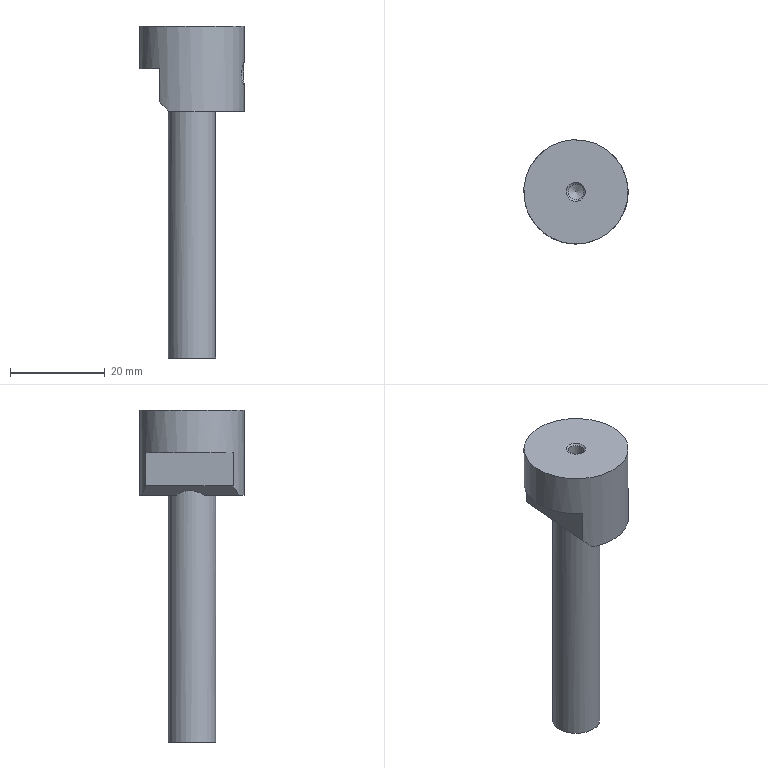Part | STEP file | SL2-MOLD_id358_xmt_txt | 1 solid | 14 faces | box 22 x 22 x 70 mm | volume 6058 mm3 | plane 7 | cylinder 5 | cone 2 | commonest cylinder face diameters 3.3 x1 5 x1 9 x1 10 x1 22 x1
STEP:
#1=CARTESIAN_POINT('',(-61.174,-74.293,77.));
#2=VERTEX_POINT('',#1);
#3=CARTESIAN_POINT('',(-61.174,-74.293,84.));
#4=VERTEX_POINT('',#3);
#5=CARTESIAN_POINT('',(-61.174,-74.293,90.));
#6=DIRECTION('',(0.,0.,1.));
#7=VECTOR('',#6,1.);
#8=LINE('',#5,#7);
#9=EDGE_CURVE('',#2,#4,#8,.T.);
#10=ORIENTED_EDGE('',*,*,#9,.F.);
#11=CARTESIAN_POINT('',(-62.781,-92.662,77.));
#12=VERTEX_POINT('',#11);
#13=CARTESIAN_POINT('',(-62.781,-92.662,77.));
#14=DIRECTION('',(-0.08716,-0.9962,0.));
#15=VECTOR('',#14,1.);
#16=LINE('',#13,#15);
#17=EDGE_CURVE('',#2,#12,#16,.T.);
#18=ORIENTED_EDGE('',*,*,#17,.T.);
#19=CARTESIAN_POINT('',(-62.781,-92.662,84.));
#20=VERTEX_POINT('',#19);
#21=CARTESIAN_POINT('',(-62.781,-92.662,90.));
#22=DIRECTION('',(0.,0.,-1.));
#23=VECTOR('',#22,1.);
#24=LINE('',#21,#23);
#25=EDGE_CURVE('',#20,#12,#24,.T.);
#26=ORIENTED_EDGE('',*,*,#25,.F.);
#27=CARTESIAN_POINT('',(-61.977,-83.477,84.));
#28=DIRECTION('',(-0.08716,-0.9962,0.));
#29=VECTOR('',#28,1.);
#30=LINE('',#27,#29);
#31=EDGE_CURVE('',#4,#20,#30,.T.);
#32=ORIENTED_EDGE('',*,*,#31,.F.);
#33=EDGE_LOOP('',(#10,#18,#26,#32));
#34=FACE_OUTER_BOUND('',#33,.T.);
#35=CARTESIAN_POINT('',(-61.977,-83.477,90.));
#36=DIRECTION('',(-0.9962,0.08716,0.));
#37=DIRECTION('',(0.,0.,-1.));
#38=AXIS2_PLACEMENT_3D('',#35,#36,#37);
#39=PLANE('',#38);
#40=ADVANCED_FACE('',(#34),#39,.T.);
#41=CARTESIAN_POINT('',(-59.092,-73.443,75.));
#42=VERTEX_POINT('',#41);
#43=CARTESIAN_POINT('',(-60.878,-93.859,75.));
#44=VERTEX_POINT('',#43);
#45=CARTESIAN_POINT('',(-56.,-84.,75.));
#46=DIRECTION('',(0.,0.,-1.));
#47=DIRECTION('',(-0.9962,0.08716,0.));
#48=AXIS2_PLACEMENT_3D('',#45,#46,#47);
#49=CIRCLE('',#48,11.);
#50=EDGE_CURVE('',#42,#44,#49,.T.);
#51=ORIENTED_EDGE('',*,*,#50,.T.);
#52=CARTESIAN_POINT('',(-60.246,-86.64,75.));
#53=VERTEX_POINT('',#52);
#54=CARTESIAN_POINT('',(-59.985,-83.651,75.));
#55=DIRECTION('',(0.08716,0.9962,0.));
#56=VECTOR('',#55,1.);
#57=LINE('',#54,#56);
#58=EDGE_CURVE('',#44,#53,#57,.T.);
#59=ORIENTED_EDGE('',*,*,#58,.T.);
#60=CARTESIAN_POINT('',(-59.723,-80.663,75.));
#61=VERTEX_POINT('',#60);
#62=CARTESIAN_POINT('',(-56.,-84.,75.));
#63=DIRECTION('',(0.,0.,1.));
#64=DIRECTION('',(-0.9962,0.08716,0.));
#65=AXIS2_PLACEMENT_3D('',#62,#63,#64);
#66=CIRCLE('',#65,5.);
#67=EDGE_CURVE('',#53,#61,#66,.T.);
#68=ORIENTED_EDGE('',*,*,#67,.T.);
#69=CARTESIAN_POINT('',(-59.985,-83.651,75.));
#70=DIRECTION('',(0.08716,0.9962,0.));
#71=VECTOR('',#70,1.);
#72=LINE('',#69,#71);
#73=EDGE_CURVE('',#61,#42,#72,.T.);
#74=ORIENTED_EDGE('',*,*,#73,.T.);
#75=EDGE_LOOP('',(#51,#59,#68,#74));
#76=FACE_OUTER_BOUND('',#75,.T.);
#77=CARTESIAN_POINT('',(-56.,-84.,75.));
#78=DIRECTION('',(0.,0.,1.));
#79=DIRECTION('',(-0.9962,0.08716,0.));
#80=AXIS2_PLACEMENT_3D('',#77,#78,#79);
#81=PLANE('',#80);
#82=ADVANCED_FACE('',(#76),#81,.F.);
#83=CARTESIAN_POINT('',(-45.115,-85.59,80.582));
#84=VERTEX_POINT('',#83);
#85=CARTESIAN_POINT('',(-45.115,-85.59,80.582));
#86=CARTESIAN_POINT('',(-45.077,-85.328,80.513));
#87=CARTESIAN_POINT('',(-45.047,-85.049,80.487));
#88=CARTESIAN_POINT('',(-45.027,-84.777,80.507));
#89=CARTESIAN_POINT('',(-45.008,-84.505,80.527));
#90=CARTESIAN_POINT('',(-45.,-84.231,80.593));
#91=CARTESIAN_POINT('',(-45.,-83.979,80.7));
#92=CARTESIAN_POINT('',(-45.,-83.726,80.807));
#93=CARTESIAN_POINT('',(-45.01,-83.488,80.958));
#94=CARTESIAN_POINT('',(-45.023,-83.282,81.141));
#95=CARTESIAN_POINT('',(-45.037,-83.073,81.328));
#96=CARTESIAN_POINT('',(-45.055,-82.892,81.553));
#97=CARTESIAN_POINT('',(-45.071,-82.756,81.798));
#98=CARTESIAN_POINT('',(-45.086,-82.618,82.045));
#99=CARTESIAN_POINT('',(-45.1,-82.522,82.32));
#100=CARTESIAN_POINT('',(-45.106,-82.476,82.599));
#101=CARTESIAN_POINT('',(-45.112,-82.431,82.872));
#102=CARTESIAN_POINT('',(-45.112,-82.433,83.157));
#103=CARTESIAN_POINT('',(-45.105,-82.481,83.43));
#104=CARTESIAN_POINT('',(-45.099,-82.529,83.698));
#105=CARTESIAN_POINT('',(-45.086,-82.623,83.962));
#106=CARTESIAN_POINT('',(-45.071,-82.755,84.2));
#107=CARTESIAN_POINT('',(-45.055,-82.889,84.442));
#108=CARTESIAN_POINT('',(-45.038,-83.066,84.664));
#109=CARTESIAN_POINT('',(-45.024,-83.271,84.849));
#110=CARTESIAN_POINT('',(-45.01,-83.481,85.038));
#111=CARTESIAN_POINT('',(-45.,-83.726,85.194));
#112=CARTESIAN_POINT('',(-45.,-83.987,85.303));
#113=CARTESIAN_POINT('',(-45.,-84.246,85.412));
#114=CARTESIAN_POINT('',(-45.009,-84.528,85.478));
#115=CARTESIAN_POINT('',(-45.03,-84.808,85.495));
#116=CARTESIAN_POINT('',(-45.05,-85.082,85.512));
#117=CARTESIAN_POINT('',(-45.081,-85.362,85.482));
#118=CARTESIAN_POINT('',(-45.121,-85.624,85.409));
#119=CARTESIAN_POINT('',(-45.16,-85.885,85.335));
#120=CARTESIAN_POINT('',(-45.207,-86.135,85.217));
#121=CARTESIAN_POINT('',(-45.255,-86.357,85.064));
#122=CARTESIAN_POINT('',(-45.305,-86.582,84.907));
#123=CARTESIAN_POINT('',(-45.357,-86.783,84.71));
#124=CARTESIAN_POINT('',(-45.401,-86.944,84.487));
#125=CARTESIAN_POINT('',(-45.447,-87.109,84.261));
#126=CARTESIAN_POINT('',(-45.487,-87.236,84.002));
#127=CARTESIAN_POINT('',(-45.512,-87.317,83.732));
#128=CARTESIAN_POINT('',(-45.537,-87.397,83.465));
#129=CARTESIAN_POINT('',(-45.549,-87.433,83.179));
#130=CARTESIAN_POINT('',(-45.546,-87.422,82.899));
#131=CARTESIAN_POINT('',(-45.542,-87.411,82.626));
#132=CARTESIAN_POINT('',(-45.524,-87.355,82.351));
#133=CARTESIAN_POINT('',(-45.494,-87.259,82.097));
#134=CARTESIAN_POINT('',(-45.464,-87.163,81.842));
#135=CARTESIAN_POINT('',(-45.422,-87.023,81.601));
#136=CARTESIAN_POINT('',(-45.376,-86.851,81.392));
#137=CARTESIAN_POINT('',(-45.329,-86.675,81.178));
#138=CARTESIAN_POINT('',(-45.276,-86.46,80.993));
#139=CARTESIAN_POINT('',(-45.227,-86.223,80.85));
#140=CARTESIAN_POINT('',(-45.187,-86.027,80.732));
#141=CARTESIAN_POINT('',(-45.148,-85.812,80.641));
#142=CARTESIAN_POINT('',(-45.115,-85.59,80.582));
#143=B_SPLINE_CURVE_WITH_KNOTS('',3,(#85,#86,#87,#88,#89,#90,#91,#92,#93,#94,#95,#96,#97,#98,#99,#100,#101,#102,#103,#104,#105,#106,#107,#108,#109,#110,#111,#112,#113,#114,#115,#116,#117,#118,#119,#120,#121,#122,#123,#124,#125,#126,#127,#128,#129,#130,#131,#132,#133,#134,#135,#136,#137,#138,#139,#140,#141,#142),.UNSPECIFIED.,.T.,.F.,(1,3,3,3,3,3,3,3,3,3,3,3,3,3,3,3,3,3,3,3,3,1),(-0.04424,0.,0.05236,0.1047,0.1573,0.2111,0.2652,0.3182,0.3704,0.4233,0.4774,0.5313,0.5839,0.6362,0.6895,0.7437,0.7973,0.8496,0.9021,0.9558,1.,1.052),.UNSPECIFIED.);
#144=EDGE_CURVE('',#84,#84,#143,.T.);
#145=ORIENTED_EDGE('',*,*,#144,.F.);
#146=EDGE_LOOP('',(#145));
#147=FACE_BOUND('',#146,.T.);
#148=ORIENTED_EDGE('',*,*,#25,.T.);
#149=CARTESIAN_POINT('',(-56.,-84.,71.));
#150=DIRECTION('',(0.7044,-0.06163,0.7071));
#151=DIRECTION('',(0.7044,-0.06163,-0.7071));
#152=AXIS2_PLACEMENT_3D('',#149,#150,#151);
#153=ELLIPSE('',#152,15.556,11.);
#154=EDGE_CURVE('',#12,#44,#153,.T.);
#155=ORIENTED_EDGE('',*,*,#154,.T.);
#156=ORIENTED_EDGE('',*,*,#50,.F.);
#157=CARTESIAN_POINT('',(-56.,-84.,71.));
#158=DIRECTION('',(0.7044,-0.06163,0.7071));
#159=DIRECTION('',(0.7044,-0.06163,-0.7071));
#160=AXIS2_PLACEMENT_3D('',#157,#158,#159);
#161=ELLIPSE('',#160,15.556,11.);
#162=EDGE_CURVE('',#42,#2,#161,.T.);
#163=ORIENTED_EDGE('',*,*,#162,.T.);
#164=ORIENTED_EDGE('',*,*,#9,.T.);
#165=CARTESIAN_POINT('',(-56.,-84.,84.));
#166=DIRECTION('',(0.,0.,-1.));
#167=DIRECTION('',(0.9962,-0.08716,0.));
#168=AXIS2_PLACEMENT_3D('',#165,#166,#167);
#169=CIRCLE('',#168,11.);
#170=EDGE_CURVE('',#20,#4,#169,.T.);
#171=ORIENTED_EDGE('',*,*,#170,.F.);
#172=EDGE_LOOP('',(#148,#155,#156,#163,#164,#171));
#173=FACE_BOUND('',#172,.T.);
#174=CARTESIAN_POINT('',(-66.958,-83.041,93.));
#175=VERTEX_POINT('',#174);
#176=CARTESIAN_POINT('',(-56.,-84.,93.));
#177=DIRECTION('',(0.,0.,-1.));
#178=DIRECTION('',(-0.9962,0.08716,0.));
#179=AXIS2_PLACEMENT_3D('',#176,#177,#178);
#180=CIRCLE('',#179,11.);
#181=EDGE_CURVE('',#175,#175,#180,.T.);
#182=ORIENTED_EDGE('',*,*,#181,.T.);
#183=EDGE_LOOP('',(#182));
#184=FACE_BOUND('',#183,.T.);
#185=CARTESIAN_POINT('',(-56.,-84.,90.));
#186=DIRECTION('',(0.,0.,-1.));
#187=DIRECTION('',(-0.9962,0.08716,0.));
#188=AXIS2_PLACEMENT_3D('',#185,#186,#187);
#189=CYLINDRICAL_SURFACE('',#188,11.);
#190=ADVANCED_FACE('',(#147,#173,#184),#189,.T.);
#191=CARTESIAN_POINT('',(-57.992,-83.826,93.));
#192=VERTEX_POINT('',#191);
#193=CARTESIAN_POINT('',(-56.,-84.,93.));
#194=DIRECTION('',(0.,0.,-1.));
#195=DIRECTION('',(-0.9962,0.08716,0.));
#196=AXIS2_PLACEMENT_3D('',#193,#194,#195);
#197=CIRCLE('',#196,2.);
#198=EDGE_CURVE('',#192,#192,#197,.T.);
#199=ORIENTED_EDGE('',*,*,#198,.T.);
#200=EDGE_LOOP('',(#199));
#201=FACE_BOUND('',#200,.T.);
#202=ORIENTED_EDGE('',*,*,#181,.F.);
#203=EDGE_LOOP('',(#202));
#204=FACE_BOUND('',#203,.T.);
#205=CARTESIAN_POINT('',(-56.,-84.,93.));
#206=DIRECTION('',(0.,0.,1.));
#207=DIRECTION('',(-0.9962,0.08716,0.));
#208=AXIS2_PLACEMENT_3D('',#205,#206,#207);
#209=PLANE('',#208);
#210=ADVANCED_FACE('',(#201,#204),#209,.T.);
#211=ORIENTED_EDGE('',*,*,#170,.T.);
#212=ORIENTED_EDGE('',*,*,#31,.T.);
#213=EDGE_LOOP('',(#211,#212));
#214=FACE_OUTER_BOUND('',#213,.T.);
#215=CARTESIAN_POINT('',(-61.977,-83.477,84.));
#216=DIRECTION('',(0.,0.,-1.));
#217=DIRECTION('',(0.9962,-0.08716,0.));
#218=AXIS2_PLACEMENT_3D('',#215,#216,#217);
#219=PLANE('',#218);
#220=ADVANCED_FACE('',(#214),#219,.T.);
#221=CARTESIAN_POINT('',(-52.49,-86.817,83.));
#222=VERTEX_POINT('',#221);
#223=CARTESIAN_POINT('',(-52.055,-81.836,83.));
#224=VERTEX_POINT('',#223);
#225=CARTESIAN_POINT('',(-52.49,-86.817,83.));
#226=CARTESIAN_POINT('',(-52.49,-86.817,82.763));
#227=CARTESIAN_POINT('',(-52.464,-86.784,82.524));
#228=CARTESIAN_POINT('',(-52.417,-86.723,82.3));
#229=CARTESIAN_POINT('',(-52.37,-86.66,82.073));
#230=CARTESIAN_POINT('',(-52.302,-86.568,81.857));
#231=CARTESIAN_POINT('',(-52.226,-86.451,81.663));
#232=CARTESIAN_POINT('',(-52.138,-86.316,81.439));
#233=CARTESIAN_POINT('',(-52.038,-86.146,81.237));
#234=CARTESIAN_POINT('',(-51.944,-85.949,81.069));
#235=CARTESIAN_POINT('',(-51.84,-85.732,80.884));
#236=CARTESIAN_POINT('',(-51.739,-85.475,80.734));
#237=CARTESIAN_POINT('',(-51.662,-85.197,80.636));
#238=CARTESIAN_POINT('',(-51.592,-84.945,80.548));
#239=CARTESIAN_POINT('',(-51.541,-84.667,80.5));
#240=CARTESIAN_POINT('',(-51.517,-84.392,80.5));
#241=CARTESIAN_POINT('',(-51.495,-84.135,80.5));
#242=CARTESIAN_POINT('',(-51.495,-83.872,80.541));
#243=CARTESIAN_POINT('',(-51.515,-83.627,80.619));
#244=CARTESIAN_POINT('',(-51.536,-83.382,80.697));
#245=CARTESIAN_POINT('',(-51.576,-83.148,80.812));
#246=CARTESIAN_POINT('',(-51.627,-82.94,80.954));
#247=CARTESIAN_POINT('',(-51.681,-82.717,81.107));
#248=CARTESIAN_POINT('',(-51.748,-82.517,81.295));
#249=CARTESIAN_POINT('',(-51.812,-82.353,81.507));
#250=CARTESIAN_POINT('',(-51.883,-82.173,81.74));
#251=CARTESIAN_POINT('',(-51.953,-82.03,82.01));
#252=CARTESIAN_POINT('',(-51.998,-81.942,82.296));
#253=CARTESIAN_POINT('',(-52.034,-81.873,82.521));
#254=CARTESIAN_POINT('',(-52.055,-81.836,82.762));
#255=CARTESIAN_POINT('',(-52.055,-81.836,83.));
#256=B_SPLINE_CURVE_WITH_KNOTS('',3,(#225,#226,#227,#228,#229,#230,#231,#232,#233,#234,#235,#236,#237,#238,#239,#240,#241,#242,#243,#244,#245,#246,#247,#248,#249,#250,#251,#252,#253,#254,#255),.UNSPECIFIED.,.F.,.F.,(4,3,3,3,3,3,3,3,3,3,4),(0.,0.08871,0.1782,0.2814,0.3957,0.4995,0.5966,0.6932,0.7966,0.9107,1.),.UNSPECIFIED.);
#257=EDGE_CURVE('',#222,#224,#256,.T.);
#258=ORIENTED_EDGE('',*,*,#257,.T.);
#259=CARTESIAN_POINT('',(-52.055,-81.836,83.));
#260=CARTESIAN_POINT('',(-52.055,-81.836,83.237));
#261=CARTESIAN_POINT('',(-52.034,-81.872,83.476));
#262=CARTESIAN_POINT('',(-51.999,-81.941,83.7));
#263=CARTESIAN_POINT('',(-51.963,-82.01,83.927));
#264=CARTESIAN_POINT('',(-51.912,-82.114,84.143));
#265=CARTESIAN_POINT('',(-51.858,-82.242,84.337));
#266=CARTESIAN_POINT('',(-51.795,-82.39,84.561));
#267=CARTESIAN_POINT('',(-51.726,-82.575,84.763));
#268=CARTESIAN_POINT('',(-51.667,-82.785,84.931));
#269=CARTESIAN_POINT('',(-51.602,-83.017,85.116));
#270=CARTESIAN_POINT('',(-51.547,-83.288,85.266));
#271=CARTESIAN_POINT('',(-51.52,-83.575,85.364));
#272=CARTESIAN_POINT('',(-51.495,-83.835,85.452));
#273=CARTESIAN_POINT('',(-51.493,-84.117,85.5));
#274=CARTESIAN_POINT('',(-51.517,-84.392,85.5));
#275=CARTESIAN_POINT('',(-51.54,-84.649,85.5));
#276=CARTESIAN_POINT('',(-51.586,-84.908,85.459));
#277=CARTESIAN_POINT('',(-51.648,-85.146,85.381));
#278=CARTESIAN_POINT('',(-51.711,-85.384,85.303));
#279=CARTESIAN_POINT('',(-51.791,-85.607,85.188));
#280=CARTESIAN_POINT('',(-51.877,-85.803,85.046));
#281=CARTESIAN_POINT('',(-51.969,-86.014,84.893));
#282=CARTESIAN_POINT('',(-52.07,-86.198,84.705));
#283=CARTESIAN_POINT('',(-52.162,-86.349,84.493));
#284=CARTESIAN_POINT('',(-52.263,-86.514,84.26));
#285=CARTESIAN_POINT('',(-52.356,-86.643,83.99));
#286=CARTESIAN_POINT('',(-52.416,-86.722,83.704));
#287=CARTESIAN_POINT('',(-52.463,-86.784,83.479));
#288=CARTESIAN_POINT('',(-52.49,-86.817,83.238));
#289=CARTESIAN_POINT('',(-52.49,-86.817,83.));
#290=B_SPLINE_CURVE_WITH_KNOTS('',3,(#259,#260,#261,#262,#263,#264,#265,#266,#267,#268,#269,#270,#271,#272,#273,#274,#275,#276,#277,#278,#279,#280,#281,#282,#283,#284,#285,#286,#287,#288,#289),.UNSPECIFIED.,.F.,.F.,(4,3,3,3,3,3,3,3,3,3,4),(0.,0.08871,0.1782,0.2814,0.3957,0.4995,0.5966,0.6932,0.7966,0.9107,1.),.UNSPECIFIED.);
#291=EDGE_CURVE('',#224,#222,#290,.T.);
#292=ORIENTED_EDGE('',*,*,#291,.T.);
#293=EDGE_LOOP('',(#258,#292));
#294=FACE_BOUND('',#293,.T.);
#295=CARTESIAN_POINT('',(-60.483,-83.608,87.));
#296=VERTEX_POINT('',#295);
#297=CARTESIAN_POINT('',(-56.,-84.,87.));
#298=DIRECTION('',(0.,0.,-1.));
#299=DIRECTION('',(-0.9962,0.08716,0.));
#300=AXIS2_PLACEMENT_3D('',#297,#298,#299);
#301=CIRCLE('',#300,4.5);
#302=EDGE_CURVE('',#296,#296,#301,.T.);
#303=ORIENTED_EDGE('',*,*,#302,.F.);
#304=EDGE_LOOP('',(#303));
#305=FACE_BOUND('',#304,.T.);
#306=CARTESIAN_POINT('',(-51.517,-84.392,23.));
#307=VERTEX_POINT('',#306);
#308=CARTESIAN_POINT('',(-56.,-84.,23.));
#309=DIRECTION('',(0.,0.,1.));
#310=DIRECTION('',(0.9962,-0.08716,0.));
#311=AXIS2_PLACEMENT_3D('',#308,#309,#310);
#312=CIRCLE('',#311,4.5);
#313=EDGE_CURVE('',#307,#307,#312,.T.);
#314=ORIENTED_EDGE('',*,*,#313,.F.);
#315=EDGE_LOOP('',(#314));
#316=FACE_BOUND('',#315,.T.);
#317=CARTESIAN_POINT('',(-56.,-84.,78.));
#318=DIRECTION('',(0.,0.,1.));
#319=DIRECTION('',(-0.9962,0.08716,0.));
#320=AXIS2_PLACEMENT_3D('',#317,#318,#319);
#321=CYLINDRICAL_SURFACE('',#320,4.5);
#322=ADVANCED_FACE('',(#294,#305,#316),#321,.F.);
#323=ORIENTED_EDGE('',*,*,#302,.T.);
#324=EDGE_LOOP('',(#323));
#325=FACE_OUTER_BOUND('',#324,.T.);
#326=CARTESIAN_POINT('',(-56.,-84.,87.));
#327=DIRECTION('',(0.,0.,1.));
#328=DIRECTION('',(-0.9962,0.08716,0.));
#329=AXIS2_PLACEMENT_3D('',#326,#327,#328);
#330=PLANE('',#329);
#331=ADVANCED_FACE('',(#325),#330,.F.);
#332=CARTESIAN_POINT('',(-54.356,-84.144,88.));
#333=VERTEX_POINT('',#332);
#334=CARTESIAN_POINT('',(-56.,-84.,88.));
#335=DIRECTION('',(0.,0.,1.));
#336=DIRECTION('',(0.9962,-0.08716,0.));
#337=AXIS2_PLACEMENT_3D('',#334,#335,#336);
#338=CIRCLE('',#337,1.65);
#339=EDGE_CURVE('',#333,#333,#338,.T.);
#340=ORIENTED_EDGE('',*,*,#339,.T.);
#341=EDGE_LOOP('',(#340));
#342=FACE_BOUND('',#341,.T.);
#343=CARTESIAN_POINT('',(-56.,-84.,87.009));
#344=VERTEX_POINT('',#343);
#345=VERTEX_LOOP('',#344);
#346=FACE_BOUND('',#345,.T.);
#347=CARTESIAN_POINT('',(-56.,-84.,88.));
#348=DIRECTION('',(0.,0.,1.));
#349=DIRECTION('',(-0.9962,0.08716,0.));
#350=AXIS2_PLACEMENT_3D('',#347,#348,#349);
#351=CONICAL_SURFACE('',#350,1.65,59.);
#352=ADVANCED_FACE('',(#342,#346),#351,.F.);
#353=CARTESIAN_POINT('',(-57.644,-83.856,92.65));
#354=VERTEX_POINT('',#353);
#355=CARTESIAN_POINT('',(-56.,-84.,92.65));
#356=DIRECTION('',(0.,0.,1.));
#357=DIRECTION('',(-0.9962,0.08716,0.));
#358=AXIS2_PLACEMENT_3D('',#355,#356,#357);
#359=CIRCLE('',#358,1.65);
#360=EDGE_CURVE('',#354,#354,#359,.T.);
#361=ORIENTED_EDGE('',*,*,#360,.T.);
#362=EDGE_LOOP('',(#361));
#363=FACE_BOUND('',#362,.T.);
#364=ORIENTED_EDGE('',*,*,#339,.F.);
#365=EDGE_LOOP('',(#364));
#366=FACE_BOUND('',#365,.T.);
#367=CARTESIAN_POINT('',(-56.,-84.,93.));
#368=DIRECTION('',(0.,0.,-1.));
#369=DIRECTION('',(0.9962,-0.08716,0.));
#370=AXIS2_PLACEMENT_3D('',#367,#368,#369);
#371=CYLINDRICAL_SURFACE('',#370,1.65);
#372=ADVANCED_FACE('',(#363,#366),#371,.F.);
#373=ORIENTED_EDGE('',*,*,#360,.F.);
#374=EDGE_LOOP('',(#373));
#375=FACE_BOUND('',#374,.T.);
#376=ORIENTED_EDGE('',*,*,#198,.F.);
#377=EDGE_LOOP('',(#376));
#378=FACE_BOUND('',#377,.T.);
#379=CARTESIAN_POINT('',(-56.,-84.,93.));
#380=DIRECTION('',(0.,0.,1.));
#381=DIRECTION('',(-0.9962,0.08716,0.));
#382=AXIS2_PLACEMENT_3D('',#379,#380,#381);
#383=CONICAL_SURFACE('',#382,2.,45.);
#384=ADVANCED_FACE('',(#375,#378),#383,.F.);
#385=ORIENTED_EDGE('',*,*,#67,.F.);
#386=CARTESIAN_POINT('',(-56.,-84.,71.));
#387=DIRECTION('',(-0.7044,0.06163,-0.7071));
#388=DIRECTION('',(0.7044,-0.06163,-0.7071));
#389=AXIS2_PLACEMENT_3D('',#386,#387,#388);
#390=ELLIPSE('',#389,7.071,5.);
#391=EDGE_CURVE('',#53,#61,#390,.T.);
#392=ORIENTED_EDGE('',*,*,#391,.T.);
#393=EDGE_LOOP('',(#385,#392));
#394=FACE_BOUND('',#393,.T.);
#395=CARTESIAN_POINT('',(-51.019,-84.436,23.));
#396=VERTEX_POINT('',#395);
#397=CARTESIAN_POINT('',(-56.,-84.,23.));
#398=DIRECTION('',(0.,0.,1.));
#399=DIRECTION('',(0.9962,-0.08716,0.));
#400=AXIS2_PLACEMENT_3D('',#397,#398,#399);
#401=CIRCLE('',#400,5.);
#402=EDGE_CURVE('',#396,#396,#401,.T.);
#403=ORIENTED_EDGE('',*,*,#402,.T.);
#404=EDGE_LOOP('',(#403));
#405=FACE_BOUND('',#404,.T.);
#406=CARTESIAN_POINT('',(-56.,-84.,90.));
#407=DIRECTION('',(0.,0.,-1.));
#408=DIRECTION('',(-0.9962,0.08716,0.));
#409=AXIS2_PLACEMENT_3D('',#406,#407,#408);
#410=CYLINDRICAL_SURFACE('',#409,5.);
#411=ADVANCED_FACE('',(#394,#405),#410,.T.);
#412=ORIENTED_EDGE('',*,*,#313,.T.);
#413=EDGE_LOOP('',(#412));
#414=FACE_BOUND('',#413,.T.);
#415=ORIENTED_EDGE('',*,*,#402,.F.);
#416=EDGE_LOOP('',(#415));
#417=FACE_BOUND('',#416,.T.);
#418=CARTESIAN_POINT('',(-56.,-84.,23.));
#419=DIRECTION('',(0.,0.,-1.));
#420=DIRECTION('',(0.9962,-0.08716,0.));
#421=AXIS2_PLACEMENT_3D('',#418,#419,#420);
#422=PLANE('',#421);
#423=ADVANCED_FACE('',(#414,#417),#422,.T.);
#424=ORIENTED_EDGE('',*,*,#144,.T.);
#425=EDGE_LOOP('',(#424));
#426=FACE_BOUND('',#425,.T.);
#427=ORIENTED_EDGE('',*,*,#291,.F.);
#428=ORIENTED_EDGE('',*,*,#257,.F.);
#429=EDGE_LOOP('',(#427,#428));
#430=FACE_BOUND('',#429,.T.);
#431=CARTESIAN_POINT('',(-56.,-84.,83.));
#432=DIRECTION('',(0.9962,-0.08716,0.));
#433=DIRECTION('',(0.,0.,1.));
#434=AXIS2_PLACEMENT_3D('',#431,#432,#433);
#435=CYLINDRICAL_SURFACE('',#434,2.5);
#436=ADVANCED_FACE('',(#426,#430),#435,.F.);
#437=ORIENTED_EDGE('',*,*,#391,.F.);
#438=ORIENTED_EDGE('',*,*,#58,.F.);
#439=ORIENTED_EDGE('',*,*,#154,.F.);
#440=ORIENTED_EDGE('',*,*,#17,.F.);
#441=ORIENTED_EDGE('',*,*,#162,.F.);
#442=ORIENTED_EDGE('',*,*,#73,.F.);
#443=EDGE_LOOP('',(#437,#438,#439,#440,#441,#442));
#444=FACE_OUTER_BOUND('',#443,.T.);
#445=CARTESIAN_POINT('',(-61.977,-83.477,77.));
#446=DIRECTION('',(-0.7044,0.06163,-0.7071));
#447=DIRECTION('',(0.08716,0.9962,0.));
#448=AXIS2_PLACEMENT_3D('',#445,#446,#447);
#449=PLANE('',#448);
#450=ADVANCED_FACE('',(#444),#449,.T.);
#451=CLOSED_SHELL('',(#40,#82,#190,#210,#220,#322,#331,#352,#372,#384,#411,#423,#436,#450));
#452=MANIFOLD_SOLID_BREP('',#451);
#453=(LENGTH_UNIT()NAMED_UNIT(*)SI_UNIT(.MILLI.,.METRE.));
#454=UNCERTAINTY_MEASURE_WITH_UNIT(LENGTH_MEASURE(0.0508),#453,'','');
#455=(NAMED_UNIT(*)PLANE_ANGLE_UNIT()SI_UNIT($,.RADIAN.));
#456=PLANE_ANGLE_MEASURE_WITH_UNIT(PLANE_ANGLE_MEASURE(0.01745),#455);
#457=DIMENSIONAL_EXPONENTS(0.,0.,0.,0.,0.,0.,0.);
#458=(CONVERSION_BASED_UNIT('DEGREE',#456)NAMED_UNIT(#457)PLANE_ANGLE_UNIT());
#459=(NAMED_UNIT(*)SI_UNIT($,.STERADIAN.)SOLID_ANGLE_UNIT());
#460=(GEOMETRIC_REPRESENTATION_CONTEXT(3)GLOBAL_UNCERTAINTY_ASSIGNED_CONTEXT((#454))GLOBAL_UNIT_ASSIGNED_CONTEXT((#453,#458,#459))REPRESENTATION_CONTEXT('',''));
#461=ADVANCED_BREP_SHAPE_REPRESENTATION('',(#452),#460);